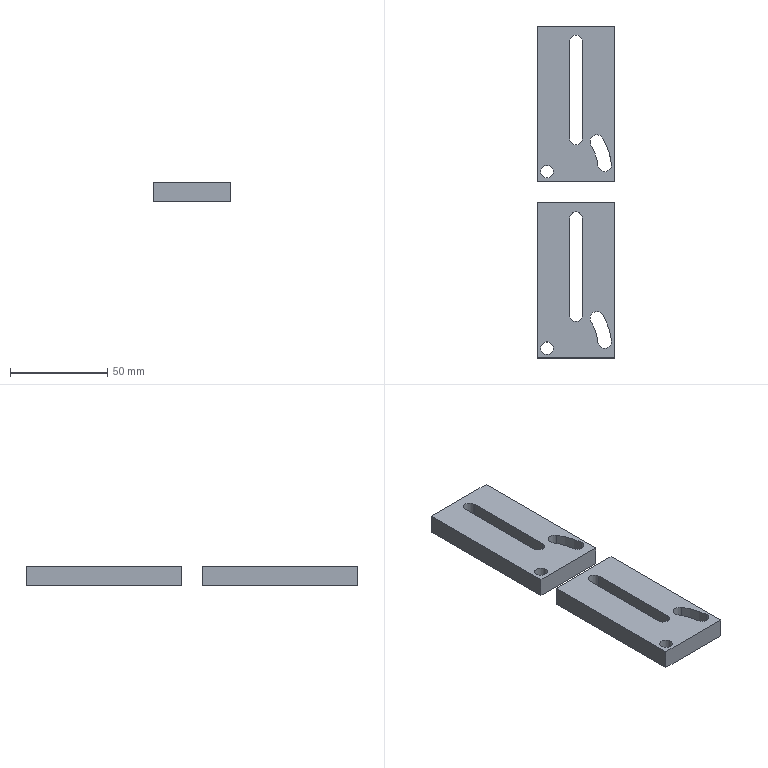Part | NX | 2 solids | 30 faces | box 40 x 171 x 10 mm | volume 53620 mm3 | plane 16 | cylinder 14 | commonest cylinder face diameters 6.5 x6 7 x4 53 x2 67 x2
STEP:
#1=CARTESIAN_POINT('',(-3.25,32.,0.));
#2=VERTEX_POINT('',#1);
#3=CARTESIAN_POINT('',(-3.25,-18.,0.));
#4=VERTEX_POINT('',#3);
#5=CARTESIAN_POINT('',(-3.25,-9.,0.));
#6=DIRECTION('',(0.,-1.,0.));
#7=VECTOR('',#6,1000.);
#8=LINE('',#5,#7);
#9=EDGE_CURVE('',#2,#4,#8,.T.);
#10=ORIENTED_EDGE('',*,*,#9,.T.);
#11=CARTESIAN_POINT('',(3.25,-18.,0.));
#12=VERTEX_POINT('',#11);
#13=CARTESIAN_POINT('',(0.,-18.,0.));
#14=DIRECTION('',(0.,0.,1.));
#15=DIRECTION('',(-1.,0.,0.));
#16=AXIS2_PLACEMENT_3D('',#13,#14,#15);
#17=CIRCLE('',#16,3.25);
#18=EDGE_CURVE('',#4,#12,#17,.T.);
#19=ORIENTED_EDGE('',*,*,#18,.T.);
#20=CARTESIAN_POINT('',(3.25,32.,0.));
#21=VERTEX_POINT('',#20);
#22=CARTESIAN_POINT('',(3.25,16.,0.));
#23=DIRECTION('',(0.,1.,0.));
#24=VECTOR('',#23,1000.);
#25=LINE('',#22,#24);
#26=EDGE_CURVE('',#12,#21,#25,.T.);
#27=ORIENTED_EDGE('',*,*,#26,.T.);
#28=CARTESIAN_POINT('',(0.,32.,0.));
#29=DIRECTION('',(0.,0.,1.));
#30=DIRECTION('',(1.,0.,0.));
#31=AXIS2_PLACEMENT_3D('',#28,#29,#30);
#32=CIRCLE('',#31,3.25);
#33=EDGE_CURVE('',#21,#2,#32,.T.);
#34=ORIENTED_EDGE('',*,*,#33,.T.);
#35=EDGE_LOOP('',(#10,#19,#27,#34));
#36=FACE_BOUND('',#35,.T.);
#37=CARTESIAN_POINT('',(-11.75,-35.,0.));
#38=VERTEX_POINT('',#37);
#39=CARTESIAN_POINT('',(-15.,-35.,0.));
#40=DIRECTION('',(0.,0.,1.));
#41=DIRECTION('',(1.,0.,0.));
#42=AXIS2_PLACEMENT_3D('',#39,#40,#41);
#43=CIRCLE('',#42,3.25);
#44=EDGE_CURVE('',#38,#38,#43,.T.);
#45=ORIENTED_EDGE('',*,*,#44,.T.);
#46=EDGE_LOOP('',(#45));
#47=FACE_BOUND('',#46,.T.);
#48=CARTESIAN_POINT('',(18.271,-31.092,0.));
#49=VERTEX_POINT('',#48);
#50=CARTESIAN_POINT('',(13.71,-17.738,0.));
#51=VERTEX_POINT('',#50);
#52=CARTESIAN_POINT('',(-15.,-35.,0.));
#53=DIRECTION('',(0.,0.,1.));
#54=DIRECTION('',(1.,0.,0.));
#55=AXIS2_PLACEMENT_3D('',#52,#53,#54);
#56=CIRCLE('',#55,33.5);
#57=EDGE_CURVE('',#49,#51,#56,.T.);
#58=ORIENTED_EDGE('',*,*,#57,.T.);
#59=CARTESIAN_POINT('',(7.711,-21.345,0.));
#60=VERTEX_POINT('',#59);
#61=CARTESIAN_POINT('',(10.711,-19.541,0.));
#62=DIRECTION('',(0.,0.,-1.));
#63=DIRECTION('',(-0.9828,0.1845,0.));
#64=AXIS2_PLACEMENT_3D('',#61,#62,#63);
#65=CIRCLE('',#64,3.5);
#66=EDGE_CURVE('',#60,#51,#65,.T.);
#67=ORIENTED_EDGE('',*,*,#66,.F.);
#68=CARTESIAN_POINT('',(11.319,-31.908,0.));
#69=VERTEX_POINT('',#68);
#70=CARTESIAN_POINT('',(-15.,-35.,0.));
#71=DIRECTION('',(0.,0.,-1.));
#72=DIRECTION('',(-1.,0.,0.));
#73=AXIS2_PLACEMENT_3D('',#70,#71,#72);
#74=CIRCLE('',#73,26.5);
#75=EDGE_CURVE('',#60,#69,#74,.T.);
#76=ORIENTED_EDGE('',*,*,#75,.T.);
#77=CARTESIAN_POINT('',(14.795,-31.5,0.));
#78=DIRECTION('',(0.,0.,-1.));
#79=DIRECTION('',(0.7472,-0.6646,0.));
#80=AXIS2_PLACEMENT_3D('',#77,#78,#79);
#81=CIRCLE('',#80,3.5);
#82=EDGE_CURVE('',#49,#69,#81,.T.);
#83=ORIENTED_EDGE('',*,*,#82,.F.);
#84=EDGE_LOOP('',(#58,#67,#76,#83));
#85=FACE_BOUND('',#84,.T.);
#86=CARTESIAN_POINT('',(20.,-40.,0.));
#87=VERTEX_POINT('',#86);
#88=CARTESIAN_POINT('',(20.,40.,0.));
#89=VERTEX_POINT('',#88);
#90=CARTESIAN_POINT('',(20.,-40.,0.));
#91=DIRECTION('',(0.,1.,0.));
#92=VECTOR('',#91,1000.);
#93=LINE('',#90,#92);
#94=EDGE_CURVE('',#87,#89,#93,.T.);
#95=ORIENTED_EDGE('',*,*,#94,.F.);
#96=CARTESIAN_POINT('',(-20.,-40.,0.));
#97=VERTEX_POINT('',#96);
#98=CARTESIAN_POINT('',(-20.,-40.,0.));
#99=DIRECTION('',(1.,0.,0.));
#100=VECTOR('',#99,1000.);
#101=LINE('',#98,#100);
#102=EDGE_CURVE('',#97,#87,#101,.T.);
#103=ORIENTED_EDGE('',*,*,#102,.F.);
#104=CARTESIAN_POINT('',(-20.,40.,0.));
#105=VERTEX_POINT('',#104);
#106=CARTESIAN_POINT('',(-20.,40.,0.));
#107=DIRECTION('',(0.,-1.,0.));
#108=VECTOR('',#107,1000.);
#109=LINE('',#106,#108);
#110=EDGE_CURVE('',#105,#97,#109,.T.);
#111=ORIENTED_EDGE('',*,*,#110,.F.);
#112=CARTESIAN_POINT('',(20.,40.,0.));
#113=DIRECTION('',(-1.,0.,0.));
#114=VECTOR('',#113,1000.);
#115=LINE('',#112,#114);
#116=EDGE_CURVE('',#89,#105,#115,.T.);
#117=ORIENTED_EDGE('',*,*,#116,.F.);
#118=EDGE_LOOP('',(#95,#103,#111,#117));
#119=FACE_BOUND('',#118,.T.);
#120=CARTESIAN_POINT('',(0.,0.,0.));
#121=DIRECTION('',(0.,0.,1.));
#122=DIRECTION('',(1.,0.,0.));
#123=AXIS2_PLACEMENT_3D('',#120,#121,#122);
#124=PLANE('',#123);
#125=ADVANCED_FACE('',(#36,#47,#85,#119),#124,.F.);
#126=CARTESIAN_POINT('',(-3.25,-18.,10.));
#127=VERTEX_POINT('',#126);
#128=CARTESIAN_POINT('',(-3.25,32.,10.));
#129=VERTEX_POINT('',#128);
#130=CARTESIAN_POINT('',(-3.25,-9.,10.));
#131=DIRECTION('',(0.,1.,0.));
#132=VECTOR('',#131,1000.);
#133=LINE('',#130,#132);
#134=EDGE_CURVE('',#127,#129,#133,.T.);
#135=ORIENTED_EDGE('',*,*,#134,.T.);
#136=CARTESIAN_POINT('',(3.25,32.,10.));
#137=VERTEX_POINT('',#136);
#138=CARTESIAN_POINT('',(0.,32.,10.));
#139=DIRECTION('',(0.,0.,-1.));
#140=DIRECTION('',(1.,0.,0.));
#141=AXIS2_PLACEMENT_3D('',#138,#139,#140);
#142=CIRCLE('',#141,3.25);
#143=EDGE_CURVE('',#129,#137,#142,.T.);
#144=ORIENTED_EDGE('',*,*,#143,.T.);
#145=CARTESIAN_POINT('',(3.25,-18.,10.));
#146=VERTEX_POINT('',#145);
#147=CARTESIAN_POINT('',(3.25,16.,10.));
#148=DIRECTION('',(0.,-1.,0.));
#149=VECTOR('',#148,1000.);
#150=LINE('',#147,#149);
#151=EDGE_CURVE('',#137,#146,#150,.T.);
#152=ORIENTED_EDGE('',*,*,#151,.T.);
#153=CARTESIAN_POINT('',(0.,-18.,10.));
#154=DIRECTION('',(0.,0.,-1.));
#155=DIRECTION('',(-1.,0.,0.));
#156=AXIS2_PLACEMENT_3D('',#153,#154,#155);
#157=CIRCLE('',#156,3.25);
#158=EDGE_CURVE('',#146,#127,#157,.T.);
#159=ORIENTED_EDGE('',*,*,#158,.T.);
#160=EDGE_LOOP('',(#135,#144,#152,#159));
#161=FACE_BOUND('',#160,.T.);
#162=CARTESIAN_POINT('',(-11.75,-35.,10.));
#163=VERTEX_POINT('',#162);
#164=CARTESIAN_POINT('',(-15.,-35.,10.));
#165=DIRECTION('',(0.,0.,-1.));
#166=DIRECTION('',(1.,0.,0.));
#167=AXIS2_PLACEMENT_3D('',#164,#165,#166);
#168=CIRCLE('',#167,3.25);
#169=EDGE_CURVE('',#163,#163,#168,.T.);
#170=ORIENTED_EDGE('',*,*,#169,.T.);
#171=EDGE_LOOP('',(#170));
#172=FACE_BOUND('',#171,.T.);
#173=CARTESIAN_POINT('',(11.319,-31.908,10.));
#174=VERTEX_POINT('',#173);
#175=CARTESIAN_POINT('',(18.271,-31.092,10.));
#176=VERTEX_POINT('',#175);
#177=CARTESIAN_POINT('',(14.795,-31.5,10.));
#178=DIRECTION('',(0.,0.,1.));
#179=DIRECTION('',(-0.6646,-0.7472,0.));
#180=AXIS2_PLACEMENT_3D('',#177,#178,#179);
#181=CIRCLE('',#180,3.5);
#182=EDGE_CURVE('',#174,#176,#181,.T.);
#183=ORIENTED_EDGE('',*,*,#182,.F.);
#184=CARTESIAN_POINT('',(7.711,-21.345,10.));
#185=VERTEX_POINT('',#184);
#186=CARTESIAN_POINT('',(-15.,-35.,10.));
#187=DIRECTION('',(0.,0.,1.));
#188=DIRECTION('',(-1.,0.,0.));
#189=AXIS2_PLACEMENT_3D('',#186,#187,#188);
#190=CIRCLE('',#189,26.5);
#191=EDGE_CURVE('',#174,#185,#190,.T.);
#192=ORIENTED_EDGE('',*,*,#191,.T.);
#193=CARTESIAN_POINT('',(13.71,-17.738,10.));
#194=VERTEX_POINT('',#193);
#195=CARTESIAN_POINT('',(10.711,-19.541,10.));
#196=DIRECTION('',(0.,0.,1.));
#197=DIRECTION('',(0.1845,0.9828,0.));
#198=AXIS2_PLACEMENT_3D('',#195,#196,#197);
#199=CIRCLE('',#198,3.5);
#200=EDGE_CURVE('',#194,#185,#199,.T.);
#201=ORIENTED_EDGE('',*,*,#200,.F.);
#202=CARTESIAN_POINT('',(-15.,-35.,10.));
#203=DIRECTION('',(0.,0.,-1.));
#204=DIRECTION('',(1.,0.,0.));
#205=AXIS2_PLACEMENT_3D('',#202,#203,#204);
#206=CIRCLE('',#205,33.5);
#207=EDGE_CURVE('',#194,#176,#206,.T.);
#208=ORIENTED_EDGE('',*,*,#207,.T.);
#209=EDGE_LOOP('',(#183,#192,#201,#208));
#210=FACE_BOUND('',#209,.T.);
#211=CARTESIAN_POINT('',(20.,-40.,10.));
#212=VERTEX_POINT('',#211);
#213=CARTESIAN_POINT('',(20.,40.,10.));
#214=VERTEX_POINT('',#213);
#215=CARTESIAN_POINT('',(20.,-40.,10.));
#216=DIRECTION('',(0.,1.,0.));
#217=VECTOR('',#216,1000.);
#218=LINE('',#215,#217);
#219=EDGE_CURVE('',#212,#214,#218,.T.);
#220=ORIENTED_EDGE('',*,*,#219,.T.);
#221=CARTESIAN_POINT('',(-20.,40.,10.));
#222=VERTEX_POINT('',#221);
#223=CARTESIAN_POINT('',(20.,40.,10.));
#224=DIRECTION('',(-1.,0.,0.));
#225=VECTOR('',#224,1000.);
#226=LINE('',#223,#225);
#227=EDGE_CURVE('',#214,#222,#226,.T.);
#228=ORIENTED_EDGE('',*,*,#227,.T.);
#229=CARTESIAN_POINT('',(-20.,-40.,10.));
#230=VERTEX_POINT('',#229);
#231=CARTESIAN_POINT('',(-20.,40.,10.));
#232=DIRECTION('',(0.,-1.,0.));
#233=VECTOR('',#232,1000.);
#234=LINE('',#231,#233);
#235=EDGE_CURVE('',#222,#230,#234,.T.);
#236=ORIENTED_EDGE('',*,*,#235,.T.);
#237=CARTESIAN_POINT('',(-20.,-40.,10.));
#238=DIRECTION('',(1.,0.,0.));
#239=VECTOR('',#238,1000.);
#240=LINE('',#237,#239);
#241=EDGE_CURVE('',#230,#212,#240,.T.);
#242=ORIENTED_EDGE('',*,*,#241,.T.);
#243=EDGE_LOOP('',(#220,#228,#236,#242));
#244=FACE_BOUND('',#243,.T.);
#245=CARTESIAN_POINT('',(0.,0.,10.));
#246=DIRECTION('',(0.,0.,1.));
#247=DIRECTION('',(1.,0.,0.));
#248=AXIS2_PLACEMENT_3D('',#245,#246,#247);
#249=PLANE('',#248);
#250=ADVANCED_FACE('',(#161,#172,#210,#244),#249,.T.);
#251=ORIENTED_EDGE('',*,*,#94,.T.);
#252=CARTESIAN_POINT('',(20.,40.,0.));
#253=DIRECTION('',(0.,0.,1.));
#254=VECTOR('',#253,1000.);
#255=LINE('',#252,#254);
#256=EDGE_CURVE('',#89,#214,#255,.T.);
#257=ORIENTED_EDGE('',*,*,#256,.T.);
#258=ORIENTED_EDGE('',*,*,#219,.F.);
#259=CARTESIAN_POINT('',(20.,-40.,0.));
#260=DIRECTION('',(0.,0.,1.));
#261=VECTOR('',#260,1000.);
#262=LINE('',#259,#261);
#263=EDGE_CURVE('',#87,#212,#262,.T.);
#264=ORIENTED_EDGE('',*,*,#263,.F.);
#265=EDGE_LOOP('',(#251,#257,#258,#264));
#266=FACE_BOUND('',#265,.T.);
#267=CARTESIAN_POINT('',(20.,-40.,0.));
#268=DIRECTION('',(1.,0.,0.));
#269=DIRECTION('',(0.,1.,0.));
#270=AXIS2_PLACEMENT_3D('',#267,#268,#269);
#271=PLANE('',#270);
#272=ADVANCED_FACE('',(#266),#271,.T.);
#273=ORIENTED_EDGE('',*,*,#116,.T.);
#274=CARTESIAN_POINT('',(-20.,40.,0.));
#275=DIRECTION('',(0.,0.,1.));
#276=VECTOR('',#275,1000.);
#277=LINE('',#274,#276);
#278=EDGE_CURVE('',#105,#222,#277,.T.);
#279=ORIENTED_EDGE('',*,*,#278,.T.);
#280=ORIENTED_EDGE('',*,*,#227,.F.);
#281=ORIENTED_EDGE('',*,*,#256,.F.);
#282=EDGE_LOOP('',(#273,#279,#280,#281));
#283=FACE_BOUND('',#282,.T.);
#284=CARTESIAN_POINT('',(20.,40.,0.));
#285=DIRECTION('',(0.,1.,0.));
#286=DIRECTION('',(-1.,0.,0.));
#287=AXIS2_PLACEMENT_3D('',#284,#285,#286);
#288=PLANE('',#287);
#289=ADVANCED_FACE('',(#283),#288,.T.);
#290=ORIENTED_EDGE('',*,*,#110,.T.);
#291=CARTESIAN_POINT('',(-20.,-40.,0.));
#292=DIRECTION('',(0.,0.,1.));
#293=VECTOR('',#292,1000.);
#294=LINE('',#291,#293);
#295=EDGE_CURVE('',#97,#230,#294,.T.);
#296=ORIENTED_EDGE('',*,*,#295,.T.);
#297=ORIENTED_EDGE('',*,*,#235,.F.);
#298=ORIENTED_EDGE('',*,*,#278,.F.);
#299=EDGE_LOOP('',(#290,#296,#297,#298));
#300=FACE_BOUND('',#299,.T.);
#301=CARTESIAN_POINT('',(-20.,40.,0.));
#302=DIRECTION('',(-1.,0.,0.));
#303=DIRECTION('',(0.,-1.,0.));
#304=AXIS2_PLACEMENT_3D('',#301,#302,#303);
#305=PLANE('',#304);
#306=ADVANCED_FACE('',(#300),#305,.T.);
#307=ORIENTED_EDGE('',*,*,#102,.T.);
#308=ORIENTED_EDGE('',*,*,#263,.T.);
#309=ORIENTED_EDGE('',*,*,#241,.F.);
#310=ORIENTED_EDGE('',*,*,#295,.F.);
#311=EDGE_LOOP('',(#307,#308,#309,#310));
#312=FACE_BOUND('',#311,.T.);
#313=CARTESIAN_POINT('',(-20.,-40.,0.));
#314=DIRECTION('',(0.,-1.,0.));
#315=DIRECTION('',(1.,0.,0.));
#316=AXIS2_PLACEMENT_3D('',#313,#314,#315);
#317=PLANE('',#316);
#318=ADVANCED_FACE('',(#312),#317,.T.);
#319=ORIENTED_EDGE('',*,*,#18,.F.);
#320=CARTESIAN_POINT('',(-3.25,-18.,10.));
#321=DIRECTION('',(0.,0.,-1.));
#322=VECTOR('',#321,1000.);
#323=LINE('',#320,#322);
#324=EDGE_CURVE('',#127,#4,#323,.T.);
#325=ORIENTED_EDGE('',*,*,#324,.F.);
#326=ORIENTED_EDGE('',*,*,#158,.F.);
#327=CARTESIAN_POINT('',(3.25,-18.,10.));
#328=DIRECTION('',(0.,0.,-1.));
#329=VECTOR('',#328,1000.);
#330=LINE('',#327,#329);
#331=EDGE_CURVE('',#146,#12,#330,.T.);
#332=ORIENTED_EDGE('',*,*,#331,.T.);
#333=EDGE_LOOP('',(#319,#325,#326,#332));
#334=FACE_BOUND('',#333,.T.);
#335=CARTESIAN_POINT('',(0.,-18.,10.));
#336=DIRECTION('',(0.,0.,-1.));
#337=DIRECTION('',(-1.,0.,0.));
#338=AXIS2_PLACEMENT_3D('',#335,#336,#337);
#339=CYLINDRICAL_SURFACE('',#338,3.25);
#340=ADVANCED_FACE('',(#334),#339,.F.);
#341=ORIENTED_EDGE('',*,*,#9,.F.);
#342=CARTESIAN_POINT('',(-3.25,32.,10.));
#343=DIRECTION('',(0.,0.,-1.));
#344=VECTOR('',#343,1000.);
#345=LINE('',#342,#344);
#346=EDGE_CURVE('',#129,#2,#345,.T.);
#347=ORIENTED_EDGE('',*,*,#346,.F.);
#348=ORIENTED_EDGE('',*,*,#134,.F.);
#349=ORIENTED_EDGE('',*,*,#324,.T.);
#350=EDGE_LOOP('',(#341,#347,#348,#349));
#351=FACE_BOUND('',#350,.T.);
#352=CARTESIAN_POINT('',(-3.25,-18.,10.));
#353=DIRECTION('',(-1.,0.,0.));
#354=DIRECTION('',(0.,1.,0.));
#355=AXIS2_PLACEMENT_3D('',#352,#353,#354);
#356=PLANE('',#355);
#357=ADVANCED_FACE('',(#351),#356,.F.);
#358=ORIENTED_EDGE('',*,*,#33,.F.);
#359=CARTESIAN_POINT('',(3.25,32.,10.));
#360=DIRECTION('',(0.,0.,-1.));
#361=VECTOR('',#360,1000.);
#362=LINE('',#359,#361);
#363=EDGE_CURVE('',#137,#21,#362,.T.);
#364=ORIENTED_EDGE('',*,*,#363,.F.);
#365=ORIENTED_EDGE('',*,*,#143,.F.);
#366=ORIENTED_EDGE('',*,*,#346,.T.);
#367=EDGE_LOOP('',(#358,#364,#365,#366));
#368=FACE_BOUND('',#367,.T.);
#369=CARTESIAN_POINT('',(0.,32.,10.));
#370=DIRECTION('',(0.,0.,-1.));
#371=DIRECTION('',(1.,0.,0.));
#372=AXIS2_PLACEMENT_3D('',#369,#370,#371);
#373=CYLINDRICAL_SURFACE('',#372,3.25);
#374=ADVANCED_FACE('',(#368),#373,.F.);
#375=ORIENTED_EDGE('',*,*,#26,.F.);
#376=ORIENTED_EDGE('',*,*,#331,.F.);
#377=ORIENTED_EDGE('',*,*,#151,.F.);
#378=ORIENTED_EDGE('',*,*,#363,.T.);
#379=EDGE_LOOP('',(#375,#376,#377,#378));
#380=FACE_BOUND('',#379,.T.);
#381=CARTESIAN_POINT('',(3.25,32.,10.));
#382=DIRECTION('',(1.,0.,0.));
#383=DIRECTION('',(0.,-1.,0.));
#384=AXIS2_PLACEMENT_3D('',#381,#382,#383);
#385=PLANE('',#384);
#386=ADVANCED_FACE('',(#380),#385,.F.);
#387=ORIENTED_EDGE('',*,*,#44,.F.);
#388=EDGE_LOOP('',(#387));
#389=FACE_BOUND('',#388,.T.);
#390=ORIENTED_EDGE('',*,*,#169,.F.);
#391=EDGE_LOOP('',(#390));
#392=FACE_BOUND('',#391,.T.);
#393=CARTESIAN_POINT('',(-15.,-35.,-80.));
#394=DIRECTION('',(0.,0.,1.));
#395=DIRECTION('',(1.,0.,0.));
#396=AXIS2_PLACEMENT_3D('',#393,#394,#395);
#397=CYLINDRICAL_SURFACE('',#396,3.25);
#398=ADVANCED_FACE('',(#389,#392),#397,.F.);
#399=CARTESIAN_POINT('',(11.319,-31.908,10.));
#400=DIRECTION('',(0.,0.,1.));
#401=VECTOR('',#400,1000.);
#402=LINE('',#399,#401);
#403=EDGE_CURVE('',#69,#174,#402,.T.);
#404=ORIENTED_EDGE('',*,*,#403,.F.);
#405=ORIENTED_EDGE('',*,*,#75,.F.);
#406=CARTESIAN_POINT('',(7.711,-21.345,10.));
#407=DIRECTION('',(0.,0.,-1.));
#408=VECTOR('',#407,1000.);
#409=LINE('',#406,#408);
#410=EDGE_CURVE('',#185,#60,#409,.T.);
#411=ORIENTED_EDGE('',*,*,#410,.F.);
#412=ORIENTED_EDGE('',*,*,#191,.F.);
#413=EDGE_LOOP('',(#404,#405,#411,#412));
#414=FACE_BOUND('',#413,.T.);
#415=CARTESIAN_POINT('',(-15.,-35.,10.));
#416=DIRECTION('',(0.,0.,-1.));
#417=DIRECTION('',(-1.,0.,0.));
#418=AXIS2_PLACEMENT_3D('',#415,#416,#417);
#419=CYLINDRICAL_SURFACE('',#418,26.5);
#420=ADVANCED_FACE('',(#414),#419,.T.);
#421=ORIENTED_EDGE('',*,*,#200,.T.);
#422=ORIENTED_EDGE('',*,*,#410,.T.);
#423=ORIENTED_EDGE('',*,*,#66,.T.);
#424=CARTESIAN_POINT('',(13.71,-17.738,10.));
#425=DIRECTION('',(0.,0.,1.));
#426=VECTOR('',#425,1000.);
#427=LINE('',#424,#426);
#428=EDGE_CURVE('',#51,#194,#427,.T.);
#429=ORIENTED_EDGE('',*,*,#428,.T.);
#430=EDGE_LOOP('',(#421,#422,#423,#429));
#431=FACE_BOUND('',#430,.T.);
#432=CARTESIAN_POINT('',(10.711,-19.541,10.));
#433=DIRECTION('',(0.,0.,-1.));
#434=DIRECTION('',(-0.9828,0.1845,0.));
#435=AXIS2_PLACEMENT_3D('',#432,#433,#434);
#436=CYLINDRICAL_SURFACE('',#435,3.5);
#437=ADVANCED_FACE('',(#431),#436,.F.);
#438=ORIENTED_EDGE('',*,*,#182,.T.);
#439=CARTESIAN_POINT('',(18.271,-31.092,10.));
#440=DIRECTION('',(0.,0.,-1.));
#441=VECTOR('',#440,1000.);
#442=LINE('',#439,#441);
#443=EDGE_CURVE('',#176,#49,#442,.T.);
#444=ORIENTED_EDGE('',*,*,#443,.T.);
#445=ORIENTED_EDGE('',*,*,#82,.T.);
#446=ORIENTED_EDGE('',*,*,#403,.T.);
#447=EDGE_LOOP('',(#438,#444,#445,#446));
#448=FACE_BOUND('',#447,.T.);
#449=CARTESIAN_POINT('',(14.795,-31.5,10.));
#450=DIRECTION('',(0.,0.,-1.));
#451=DIRECTION('',(-0.6646,-0.7472,0.));
#452=AXIS2_PLACEMENT_3D('',#449,#450,#451);
#453=CYLINDRICAL_SURFACE('',#452,3.5);
#454=ADVANCED_FACE('',(#448),#453,.F.);
#455=ORIENTED_EDGE('',*,*,#443,.F.);
#456=ORIENTED_EDGE('',*,*,#207,.F.);
#457=ORIENTED_EDGE('',*,*,#428,.F.);
#458=ORIENTED_EDGE('',*,*,#57,.F.);
#459=EDGE_LOOP('',(#455,#456,#457,#458));
#460=FACE_BOUND('',#459,.T.);
#461=CARTESIAN_POINT('',(-15.,-35.,10.));
#462=DIRECTION('',(0.,0.,-1.));
#463=DIRECTION('',(1.,0.,0.));
#464=AXIS2_PLACEMENT_3D('',#461,#462,#463);
#465=CYLINDRICAL_SURFACE('',#464,33.5);
#466=ADVANCED_FACE('',(#460),#465,.F.);
#467=CLOSED_SHELL('',(#125,#250,#272,#289,#306,#318,#340,#357,#374,#386,#398,#420,#437,#454,#466));
#468=MANIFOLD_SOLID_BREP('',#467);
#469=CARTESIAN_POINT('',(-3.25,-59.,0.));
#470=VERTEX_POINT('',#469);
#471=CARTESIAN_POINT('',(-3.25,-109.,0.));
#472=VERTEX_POINT('',#471);
#473=CARTESIAN_POINT('',(-3.25,-100.,0.));
#474=DIRECTION('',(0.,-1.,0.));
#475=VECTOR('',#474,1000.);
#476=LINE('',#473,#475);
#477=EDGE_CURVE('',#470,#472,#476,.T.);
#478=ORIENTED_EDGE('',*,*,#477,.T.);
#479=CARTESIAN_POINT('',(3.25,-109.,0.));
#480=VERTEX_POINT('',#479);
#481=CARTESIAN_POINT('',(0.,-109.,0.));
#482=DIRECTION('',(0.,0.,1.));
#483=DIRECTION('',(-1.,0.,0.));
#484=AXIS2_PLACEMENT_3D('',#481,#482,#483);
#485=CIRCLE('',#484,3.25);
#486=EDGE_CURVE('',#472,#480,#485,.T.);
#487=ORIENTED_EDGE('',*,*,#486,.T.);
#488=CARTESIAN_POINT('',(3.25,-59.,0.));
#489=VERTEX_POINT('',#488);
#490=CARTESIAN_POINT('',(3.25,-75.,0.));
#491=DIRECTION('',(0.,1.,0.));
#492=VECTOR('',#491,1000.);
#493=LINE('',#490,#492);
#494=EDGE_CURVE('',#480,#489,#493,.T.);
#495=ORIENTED_EDGE('',*,*,#494,.T.);
#496=CARTESIAN_POINT('',(0.,-59.,0.));
#497=DIRECTION('',(0.,0.,1.));
#498=DIRECTION('',(1.,0.,0.));
#499=AXIS2_PLACEMENT_3D('',#496,#497,#498);
#500=CIRCLE('',#499,3.25);
#501=EDGE_CURVE('',#489,#470,#500,.T.);
#502=ORIENTED_EDGE('',*,*,#501,.T.);
#503=EDGE_LOOP('',(#478,#487,#495,#502));
#504=FACE_BOUND('',#503,.T.);
#505=CARTESIAN_POINT('',(-11.75,-126.,0.));
#506=VERTEX_POINT('',#505);
#507=CARTESIAN_POINT('',(-15.,-126.,0.));
#508=DIRECTION('',(0.,0.,1.));
#509=DIRECTION('',(1.,0.,0.));
#510=AXIS2_PLACEMENT_3D('',#507,#508,#509);
#511=CIRCLE('',#510,3.25);
#512=EDGE_CURVE('',#506,#506,#511,.T.);
#513=ORIENTED_EDGE('',*,*,#512,.T.);
#514=EDGE_LOOP('',(#513));
#515=FACE_BOUND('',#514,.T.);
#516=CARTESIAN_POINT('',(18.271,-122.092,0.));
#517=VERTEX_POINT('',#516);
#518=CARTESIAN_POINT('',(13.71,-108.738,0.));
#519=VERTEX_POINT('',#518);
#520=CARTESIAN_POINT('',(-15.,-126.,0.));
#521=DIRECTION('',(0.,0.,1.));
#522=DIRECTION('',(1.,0.,0.));
#523=AXIS2_PLACEMENT_3D('',#520,#521,#522);
#524=CIRCLE('',#523,33.5);
#525=EDGE_CURVE('',#517,#519,#524,.T.);
#526=ORIENTED_EDGE('',*,*,#525,.T.);
#527=CARTESIAN_POINT('',(7.711,-112.345,0.));
#528=VERTEX_POINT('',#527);
#529=CARTESIAN_POINT('',(10.711,-110.541,0.));
#530=DIRECTION('',(0.,0.,-1.));
#531=DIRECTION('',(-0.9828,0.1845,0.));
#532=AXIS2_PLACEMENT_3D('',#529,#530,#531);
#533=CIRCLE('',#532,3.5);
#534=EDGE_CURVE('',#528,#519,#533,.T.);
#535=ORIENTED_EDGE('',*,*,#534,.F.);
#536=CARTESIAN_POINT('',(11.319,-122.908,0.));
#537=VERTEX_POINT('',#536);
#538=CARTESIAN_POINT('',(-15.,-126.,0.));
#539=DIRECTION('',(0.,0.,-1.));
#540=DIRECTION('',(-1.,0.,0.));
#541=AXIS2_PLACEMENT_3D('',#538,#539,#540);
#542=CIRCLE('',#541,26.5);
#543=EDGE_CURVE('',#528,#537,#542,.T.);
#544=ORIENTED_EDGE('',*,*,#543,.T.);
#545=CARTESIAN_POINT('',(14.795,-122.5,0.));
#546=DIRECTION('',(0.,0.,-1.));
#547=DIRECTION('',(0.7472,-0.6646,0.));
#548=AXIS2_PLACEMENT_3D('',#545,#546,#547);
#549=CIRCLE('',#548,3.5);
#550=EDGE_CURVE('',#517,#537,#549,.T.);
#551=ORIENTED_EDGE('',*,*,#550,.F.);
#552=EDGE_LOOP('',(#526,#535,#544,#551));
#553=FACE_BOUND('',#552,.T.);
#554=CARTESIAN_POINT('',(20.,-131.,0.));
#555=VERTEX_POINT('',#554);
#556=CARTESIAN_POINT('',(20.,-51.,0.));
#557=VERTEX_POINT('',#556);
#558=CARTESIAN_POINT('',(20.,-131.,0.));
#559=DIRECTION('',(0.,1.,0.));
#560=VECTOR('',#559,1000.);
#561=LINE('',#558,#560);
#562=EDGE_CURVE('',#555,#557,#561,.T.);
#563=ORIENTED_EDGE('',*,*,#562,.F.);
#564=CARTESIAN_POINT('',(-20.,-131.,0.));
#565=VERTEX_POINT('',#564);
#566=CARTESIAN_POINT('',(-20.,-131.,0.));
#567=DIRECTION('',(1.,0.,0.));
#568=VECTOR('',#567,1000.);
#569=LINE('',#566,#568);
#570=EDGE_CURVE('',#565,#555,#569,.T.);
#571=ORIENTED_EDGE('',*,*,#570,.F.);
#572=CARTESIAN_POINT('',(-20.,-51.,0.));
#573=VERTEX_POINT('',#572);
#574=CARTESIAN_POINT('',(-20.,-51.,0.));
#575=DIRECTION('',(0.,-1.,0.));
#576=VECTOR('',#575,1000.);
#577=LINE('',#574,#576);
#578=EDGE_CURVE('',#573,#565,#577,.T.);
#579=ORIENTED_EDGE('',*,*,#578,.F.);
#580=CARTESIAN_POINT('',(20.,-51.,0.));
#581=DIRECTION('',(-1.,0.,0.));
#582=VECTOR('',#581,1000.);
#583=LINE('',#580,#582);
#584=EDGE_CURVE('',#557,#573,#583,.T.);
#585=ORIENTED_EDGE('',*,*,#584,.F.);
#586=EDGE_LOOP('',(#563,#571,#579,#585));
#587=FACE_BOUND('',#586,.T.);
#588=CARTESIAN_POINT('',(0.,-91.,0.));
#589=DIRECTION('',(0.,0.,1.));
#590=DIRECTION('',(1.,0.,0.));
#591=AXIS2_PLACEMENT_3D('',#588,#589,#590);
#592=PLANE('',#591);
#593=ADVANCED_FACE('',(#504,#515,#553,#587),#592,.F.);
#594=CARTESIAN_POINT('',(-3.25,-109.,10.));
#595=VERTEX_POINT('',#594);
#596=CARTESIAN_POINT('',(-3.25,-59.,10.));
#597=VERTEX_POINT('',#596);
#598=CARTESIAN_POINT('',(-3.25,-100.,10.));
#599=DIRECTION('',(0.,1.,0.));
#600=VECTOR('',#599,1000.);
#601=LINE('',#598,#600);
#602=EDGE_CURVE('',#595,#597,#601,.T.);
#603=ORIENTED_EDGE('',*,*,#602,.T.);
#604=CARTESIAN_POINT('',(3.25,-59.,10.));
#605=VERTEX_POINT('',#604);
#606=CARTESIAN_POINT('',(0.,-59.,10.));
#607=DIRECTION('',(0.,0.,-1.));
#608=DIRECTION('',(1.,0.,0.));
#609=AXIS2_PLACEMENT_3D('',#606,#607,#608);
#610=CIRCLE('',#609,3.25);
#611=EDGE_CURVE('',#597,#605,#610,.T.);
#612=ORIENTED_EDGE('',*,*,#611,.T.);
#613=CARTESIAN_POINT('',(3.25,-109.,10.));
#614=VERTEX_POINT('',#613);
#615=CARTESIAN_POINT('',(3.25,-75.,10.));
#616=DIRECTION('',(0.,-1.,0.));
#617=VECTOR('',#616,1000.);
#618=LINE('',#615,#617);
#619=EDGE_CURVE('',#605,#614,#618,.T.);
#620=ORIENTED_EDGE('',*,*,#619,.T.);
#621=CARTESIAN_POINT('',(0.,-109.,10.));
#622=DIRECTION('',(0.,0.,-1.));
#623=DIRECTION('',(-1.,0.,0.));
#624=AXIS2_PLACEMENT_3D('',#621,#622,#623);
#625=CIRCLE('',#624,3.25);
#626=EDGE_CURVE('',#614,#595,#625,.T.);
#627=ORIENTED_EDGE('',*,*,#626,.T.);
#628=EDGE_LOOP('',(#603,#612,#620,#627));
#629=FACE_BOUND('',#628,.T.);
#630=CARTESIAN_POINT('',(-11.75,-126.,10.));
#631=VERTEX_POINT('',#630);
#632=CARTESIAN_POINT('',(-15.,-126.,10.));
#633=DIRECTION('',(0.,0.,-1.));
#634=DIRECTION('',(1.,0.,0.));
#635=AXIS2_PLACEMENT_3D('',#632,#633,#634);
#636=CIRCLE('',#635,3.25);
#637=EDGE_CURVE('',#631,#631,#636,.T.);
#638=ORIENTED_EDGE('',*,*,#637,.T.);
#639=EDGE_LOOP('',(#638));
#640=FACE_BOUND('',#639,.T.);
#641=CARTESIAN_POINT('',(11.319,-122.908,10.));
#642=VERTEX_POINT('',#641);
#643=CARTESIAN_POINT('',(18.271,-122.092,10.));
#644=VERTEX_POINT('',#643);
#645=CARTESIAN_POINT('',(14.795,-122.5,10.));
#646=DIRECTION('',(0.,0.,1.));
#647=DIRECTION('',(-0.6646,-0.7472,0.));
#648=AXIS2_PLACEMENT_3D('',#645,#646,#647);
#649=CIRCLE('',#648,3.5);
#650=EDGE_CURVE('',#642,#644,#649,.T.);
#651=ORIENTED_EDGE('',*,*,#650,.F.);
#652=CARTESIAN_POINT('',(7.711,-112.345,10.));
#653=VERTEX_POINT('',#652);
#654=CARTESIAN_POINT('',(-15.,-126.,10.));
#655=DIRECTION('',(0.,0.,1.));
#656=DIRECTION('',(-1.,0.,0.));
#657=AXIS2_PLACEMENT_3D('',#654,#655,#656);
#658=CIRCLE('',#657,26.5);
#659=EDGE_CURVE('',#642,#653,#658,.T.);
#660=ORIENTED_EDGE('',*,*,#659,.T.);
#661=CARTESIAN_POINT('',(13.71,-108.738,10.));
#662=VERTEX_POINT('',#661);
#663=CARTESIAN_POINT('',(10.711,-110.541,10.));
#664=DIRECTION('',(0.,0.,1.));
#665=DIRECTION('',(0.1845,0.9828,0.));
#666=AXIS2_PLACEMENT_3D('',#663,#664,#665);
#667=CIRCLE('',#666,3.5);
#668=EDGE_CURVE('',#662,#653,#667,.T.);
#669=ORIENTED_EDGE('',*,*,#668,.F.);
#670=CARTESIAN_POINT('',(-15.,-126.,10.));
#671=DIRECTION('',(0.,0.,-1.));
#672=DIRECTION('',(1.,0.,0.));
#673=AXIS2_PLACEMENT_3D('',#670,#671,#672);
#674=CIRCLE('',#673,33.5);
#675=EDGE_CURVE('',#662,#644,#674,.T.);
#676=ORIENTED_EDGE('',*,*,#675,.T.);
#677=EDGE_LOOP('',(#651,#660,#669,#676));
#678=FACE_BOUND('',#677,.T.);
#679=CARTESIAN_POINT('',(20.,-131.,10.));
#680=VERTEX_POINT('',#679);
#681=CARTESIAN_POINT('',(20.,-51.,10.));
#682=VERTEX_POINT('',#681);
#683=CARTESIAN_POINT('',(20.,-131.,10.));
#684=DIRECTION('',(0.,1.,0.));
#685=VECTOR('',#684,1000.);
#686=LINE('',#683,#685);
#687=EDGE_CURVE('',#680,#682,#686,.T.);
#688=ORIENTED_EDGE('',*,*,#687,.T.);
#689=CARTESIAN_POINT('',(-20.,-51.,10.));
#690=VERTEX_POINT('',#689);
#691=CARTESIAN_POINT('',(20.,-51.,10.));
#692=DIRECTION('',(-1.,0.,0.));
#693=VECTOR('',#692,1000.);
#694=LINE('',#691,#693);
#695=EDGE_CURVE('',#682,#690,#694,.T.);
#696=ORIENTED_EDGE('',*,*,#695,.T.);
#697=CARTESIAN_POINT('',(-20.,-131.,10.));
#698=VERTEX_POINT('',#697);
#699=CARTESIAN_POINT('',(-20.,-51.,10.));
#700=DIRECTION('',(0.,-1.,0.));
#701=VECTOR('',#700,1000.);
#702=LINE('',#699,#701);
#703=EDGE_CURVE('',#690,#698,#702,.T.);
#704=ORIENTED_EDGE('',*,*,#703,.T.);
#705=CARTESIAN_POINT('',(-20.,-131.,10.));
#706=DIRECTION('',(1.,0.,0.));
#707=VECTOR('',#706,1000.);
#708=LINE('',#705,#707);
#709=EDGE_CURVE('',#698,#680,#708,.T.);
#710=ORIENTED_EDGE('',*,*,#709,.T.);
#711=EDGE_LOOP('',(#688,#696,#704,#710));
#712=FACE_BOUND('',#711,.T.);
#713=CARTESIAN_POINT('',(0.,-91.,10.));
#714=DIRECTION('',(0.,0.,1.));
#715=DIRECTION('',(1.,0.,0.));
#716=AXIS2_PLACEMENT_3D('',#713,#714,#715);
#717=PLANE('',#716);
#718=ADVANCED_FACE('',(#629,#640,#678,#712),#717,.T.);
#719=ORIENTED_EDGE('',*,*,#562,.T.);
#720=CARTESIAN_POINT('',(20.,-51.,0.));
#721=DIRECTION('',(0.,0.,1.));
#722=VECTOR('',#721,1000.);
#723=LINE('',#720,#722);
#724=EDGE_CURVE('',#557,#682,#723,.T.);
#725=ORIENTED_EDGE('',*,*,#724,.T.);
#726=ORIENTED_EDGE('',*,*,#687,.F.);
#727=CARTESIAN_POINT('',(20.,-131.,0.));
#728=DIRECTION('',(0.,0.,1.));
#729=VECTOR('',#728,1000.);
#730=LINE('',#727,#729);
#731=EDGE_CURVE('',#555,#680,#730,.T.);
#732=ORIENTED_EDGE('',*,*,#731,.F.);
#733=EDGE_LOOP('',(#719,#725,#726,#732));
#734=FACE_BOUND('',#733,.T.);
#735=CARTESIAN_POINT('',(20.,-131.,0.));
#736=DIRECTION('',(1.,0.,0.));
#737=DIRECTION('',(0.,1.,0.));
#738=AXIS2_PLACEMENT_3D('',#735,#736,#737);
#739=PLANE('',#738);
#740=ADVANCED_FACE('',(#734),#739,.T.);
#741=ORIENTED_EDGE('',*,*,#584,.T.);
#742=CARTESIAN_POINT('',(-20.,-51.,0.));
#743=DIRECTION('',(0.,0.,1.));
#744=VECTOR('',#743,1000.);
#745=LINE('',#742,#744);
#746=EDGE_CURVE('',#573,#690,#745,.T.);
#747=ORIENTED_EDGE('',*,*,#746,.T.);
#748=ORIENTED_EDGE('',*,*,#695,.F.);
#749=ORIENTED_EDGE('',*,*,#724,.F.);
#750=EDGE_LOOP('',(#741,#747,#748,#749));
#751=FACE_BOUND('',#750,.T.);
#752=CARTESIAN_POINT('',(20.,-51.,0.));
#753=DIRECTION('',(0.,1.,0.));
#754=DIRECTION('',(-1.,0.,0.));
#755=AXIS2_PLACEMENT_3D('',#752,#753,#754);
#756=PLANE('',#755);
#757=ADVANCED_FACE('',(#751),#756,.T.);
#758=ORIENTED_EDGE('',*,*,#578,.T.);
#759=CARTESIAN_POINT('',(-20.,-131.,0.));
#760=DIRECTION('',(0.,0.,1.));
#761=VECTOR('',#760,1000.);
#762=LINE('',#759,#761);
#763=EDGE_CURVE('',#565,#698,#762,.T.);
#764=ORIENTED_EDGE('',*,*,#763,.T.);
#765=ORIENTED_EDGE('',*,*,#703,.F.);
#766=ORIENTED_EDGE('',*,*,#746,.F.);
#767=EDGE_LOOP('',(#758,#764,#765,#766));
#768=FACE_BOUND('',#767,.T.);
#769=CARTESIAN_POINT('',(-20.,-51.,0.));
#770=DIRECTION('',(-1.,0.,0.));
#771=DIRECTION('',(0.,-1.,0.));
#772=AXIS2_PLACEMENT_3D('',#769,#770,#771);
#773=PLANE('',#772);
#774=ADVANCED_FACE('',(#768),#773,.T.);
#775=ORIENTED_EDGE('',*,*,#570,.T.);
#776=ORIENTED_EDGE('',*,*,#731,.T.);
#777=ORIENTED_EDGE('',*,*,#709,.F.);
#778=ORIENTED_EDGE('',*,*,#763,.F.);
#779=EDGE_LOOP('',(#775,#776,#777,#778));
#780=FACE_BOUND('',#779,.T.);
#781=CARTESIAN_POINT('',(-20.,-131.,0.));
#782=DIRECTION('',(0.,-1.,0.));
#783=DIRECTION('',(1.,0.,0.));
#784=AXIS2_PLACEMENT_3D('',#781,#782,#783);
#785=PLANE('',#784);
#786=ADVANCED_FACE('',(#780),#785,.T.);
#787=ORIENTED_EDGE('',*,*,#486,.F.);
#788=CARTESIAN_POINT('',(-3.25,-109.,10.));
#789=DIRECTION('',(0.,0.,-1.));
#790=VECTOR('',#789,1000.);
#791=LINE('',#788,#790);
#792=EDGE_CURVE('',#595,#472,#791,.T.);
#793=ORIENTED_EDGE('',*,*,#792,.F.);
#794=ORIENTED_EDGE('',*,*,#626,.F.);
#795=CARTESIAN_POINT('',(3.25,-109.,10.));
#796=DIRECTION('',(0.,0.,-1.));
#797=VECTOR('',#796,1000.);
#798=LINE('',#795,#797);
#799=EDGE_CURVE('',#614,#480,#798,.T.);
#800=ORIENTED_EDGE('',*,*,#799,.T.);
#801=EDGE_LOOP('',(#787,#793,#794,#800));
#802=FACE_BOUND('',#801,.T.);
#803=CARTESIAN_POINT('',(0.,-109.,10.));
#804=DIRECTION('',(0.,0.,-1.));
#805=DIRECTION('',(-1.,0.,0.));
#806=AXIS2_PLACEMENT_3D('',#803,#804,#805);
#807=CYLINDRICAL_SURFACE('',#806,3.25);
#808=ADVANCED_FACE('',(#802),#807,.F.);
#809=ORIENTED_EDGE('',*,*,#477,.F.);
#810=CARTESIAN_POINT('',(-3.25,-59.,10.));
#811=DIRECTION('',(0.,0.,-1.));
#812=VECTOR('',#811,1000.);
#813=LINE('',#810,#812);
#814=EDGE_CURVE('',#597,#470,#813,.T.);
#815=ORIENTED_EDGE('',*,*,#814,.F.);
#816=ORIENTED_EDGE('',*,*,#602,.F.);
#817=ORIENTED_EDGE('',*,*,#792,.T.);
#818=EDGE_LOOP('',(#809,#815,#816,#817));
#819=FACE_BOUND('',#818,.T.);
#820=CARTESIAN_POINT('',(-3.25,-109.,10.));
#821=DIRECTION('',(-1.,0.,0.));
#822=DIRECTION('',(0.,1.,0.));
#823=AXIS2_PLACEMENT_3D('',#820,#821,#822);
#824=PLANE('',#823);
#825=ADVANCED_FACE('',(#819),#824,.F.);
#826=ORIENTED_EDGE('',*,*,#501,.F.);
#827=CARTESIAN_POINT('',(3.25,-59.,10.));
#828=DIRECTION('',(0.,0.,-1.));
#829=VECTOR('',#828,1000.);
#830=LINE('',#827,#829);
#831=EDGE_CURVE('',#605,#489,#830,.T.);
#832=ORIENTED_EDGE('',*,*,#831,.F.);
#833=ORIENTED_EDGE('',*,*,#611,.F.);
#834=ORIENTED_EDGE('',*,*,#814,.T.);
#835=EDGE_LOOP('',(#826,#832,#833,#834));
#836=FACE_BOUND('',#835,.T.);
#837=CARTESIAN_POINT('',(0.,-59.,10.));
#838=DIRECTION('',(0.,0.,-1.));
#839=DIRECTION('',(1.,0.,0.));
#840=AXIS2_PLACEMENT_3D('',#837,#838,#839);
#841=CYLINDRICAL_SURFACE('',#840,3.25);
#842=ADVANCED_FACE('',(#836),#841,.F.);
#843=ORIENTED_EDGE('',*,*,#494,.F.);
#844=ORIENTED_EDGE('',*,*,#799,.F.);
#845=ORIENTED_EDGE('',*,*,#619,.F.);
#846=ORIENTED_EDGE('',*,*,#831,.T.);
#847=EDGE_LOOP('',(#843,#844,#845,#846));
#848=FACE_BOUND('',#847,.T.);
#849=CARTESIAN_POINT('',(3.25,-59.,10.));
#850=DIRECTION('',(1.,0.,0.));
#851=DIRECTION('',(0.,-1.,0.));
#852=AXIS2_PLACEMENT_3D('',#849,#850,#851);
#853=PLANE('',#852);
#854=ADVANCED_FACE('',(#848),#853,.F.);
#855=ORIENTED_EDGE('',*,*,#512,.F.);
#856=EDGE_LOOP('',(#855));
#857=FACE_BOUND('',#856,.T.);
#858=ORIENTED_EDGE('',*,*,#637,.F.);
#859=EDGE_LOOP('',(#858));
#860=FACE_BOUND('',#859,.T.);
#861=CARTESIAN_POINT('',(-15.,-126.,-80.));
#862=DIRECTION('',(0.,0.,1.));
#863=DIRECTION('',(1.,0.,0.));
#864=AXIS2_PLACEMENT_3D('',#861,#862,#863);
#865=CYLINDRICAL_SURFACE('',#864,3.25);
#866=ADVANCED_FACE('',(#857,#860),#865,.F.);
#867=CARTESIAN_POINT('',(11.319,-122.908,10.));
#868=DIRECTION('',(0.,0.,1.));
#869=VECTOR('',#868,1000.);
#870=LINE('',#867,#869);
#871=EDGE_CURVE('',#537,#642,#870,.T.);
#872=ORIENTED_EDGE('',*,*,#871,.F.);
#873=ORIENTED_EDGE('',*,*,#543,.F.);
#874=CARTESIAN_POINT('',(7.711,-112.345,10.));
#875=DIRECTION('',(0.,0.,-1.));
#876=VECTOR('',#875,1000.);
#877=LINE('',#874,#876);
#878=EDGE_CURVE('',#653,#528,#877,.T.);
#879=ORIENTED_EDGE('',*,*,#878,.F.);
#880=ORIENTED_EDGE('',*,*,#659,.F.);
#881=EDGE_LOOP('',(#872,#873,#879,#880));
#882=FACE_BOUND('',#881,.T.);
#883=CARTESIAN_POINT('',(-15.,-126.,10.));
#884=DIRECTION('',(0.,0.,-1.));
#885=DIRECTION('',(-1.,0.,0.));
#886=AXIS2_PLACEMENT_3D('',#883,#884,#885);
#887=CYLINDRICAL_SURFACE('',#886,26.5);
#888=ADVANCED_FACE('',(#882),#887,.T.);
#889=ORIENTED_EDGE('',*,*,#668,.T.);
#890=ORIENTED_EDGE('',*,*,#878,.T.);
#891=ORIENTED_EDGE('',*,*,#534,.T.);
#892=CARTESIAN_POINT('',(13.71,-108.738,10.));
#893=DIRECTION('',(0.,0.,1.));
#894=VECTOR('',#893,1000.);
#895=LINE('',#892,#894);
#896=EDGE_CURVE('',#519,#662,#895,.T.);
#897=ORIENTED_EDGE('',*,*,#896,.T.);
#898=EDGE_LOOP('',(#889,#890,#891,#897));
#899=FACE_BOUND('',#898,.T.);
#900=CARTESIAN_POINT('',(10.711,-110.541,10.));
#901=DIRECTION('',(0.,0.,-1.));
#902=DIRECTION('',(-0.9828,0.1845,0.));
#903=AXIS2_PLACEMENT_3D('',#900,#901,#902);
#904=CYLINDRICAL_SURFACE('',#903,3.5);
#905=ADVANCED_FACE('',(#899),#904,.F.);
#906=ORIENTED_EDGE('',*,*,#650,.T.);
#907=CARTESIAN_POINT('',(18.271,-122.092,10.));
#908=DIRECTION('',(0.,0.,-1.));
#909=VECTOR('',#908,1000.);
#910=LINE('',#907,#909);
#911=EDGE_CURVE('',#644,#517,#910,.T.);
#912=ORIENTED_EDGE('',*,*,#911,.T.);
#913=ORIENTED_EDGE('',*,*,#550,.T.);
#914=ORIENTED_EDGE('',*,*,#871,.T.);
#915=EDGE_LOOP('',(#906,#912,#913,#914));
#916=FACE_BOUND('',#915,.T.);
#917=CARTESIAN_POINT('',(14.795,-122.5,10.));
#918=DIRECTION('',(0.,0.,-1.));
#919=DIRECTION('',(-0.6646,-0.7472,0.));
#920=AXIS2_PLACEMENT_3D('',#917,#918,#919);
#921=CYLINDRICAL_SURFACE('',#920,3.5);
#922=ADVANCED_FACE('',(#916),#921,.F.);
#923=ORIENTED_EDGE('',*,*,#911,.F.);
#924=ORIENTED_EDGE('',*,*,#675,.F.);
#925=ORIENTED_EDGE('',*,*,#896,.F.);
#926=ORIENTED_EDGE('',*,*,#525,.F.);
#927=EDGE_LOOP('',(#923,#924,#925,#926));
#928=FACE_BOUND('',#927,.T.);
#929=CARTESIAN_POINT('',(-15.,-126.,10.));
#930=DIRECTION('',(0.,0.,-1.));
#931=DIRECTION('',(1.,0.,0.));
#932=AXIS2_PLACEMENT_3D('',#929,#930,#931);
#933=CYLINDRICAL_SURFACE('',#932,33.5);
#934=ADVANCED_FACE('',(#928),#933,.F.);
#935=CLOSED_SHELL('',(#593,#718,#740,#757,#774,#786,#808,#825,#842,#854,#866,#888,#905,#922,#934));
#936=MANIFOLD_SOLID_BREP('',#935);
#937=(LENGTH_UNIT()NAMED_UNIT(*)SI_UNIT(.MILLI.,.METRE.));
#938=UNCERTAINTY_MEASURE_WITH_UNIT(LENGTH_MEASURE(0.00001),#937,'','');
#939=(NAMED_UNIT(*)PLANE_ANGLE_UNIT()SI_UNIT($,.RADIAN.));
#940=(NAMED_UNIT(*)SI_UNIT($,.STERADIAN.)SOLID_ANGLE_UNIT());
#941=(GEOMETRIC_REPRESENTATION_CONTEXT(3)GLOBAL_UNCERTAINTY_ASSIGNED_CONTEXT((#938))GLOBAL_UNIT_ASSIGNED_CONTEXT((#937,#939,#940))REPRESENTATION_CONTEXT('',''));
#942=ADVANCED_BREP_SHAPE_REPRESENTATION('',(#468,#936),#941);